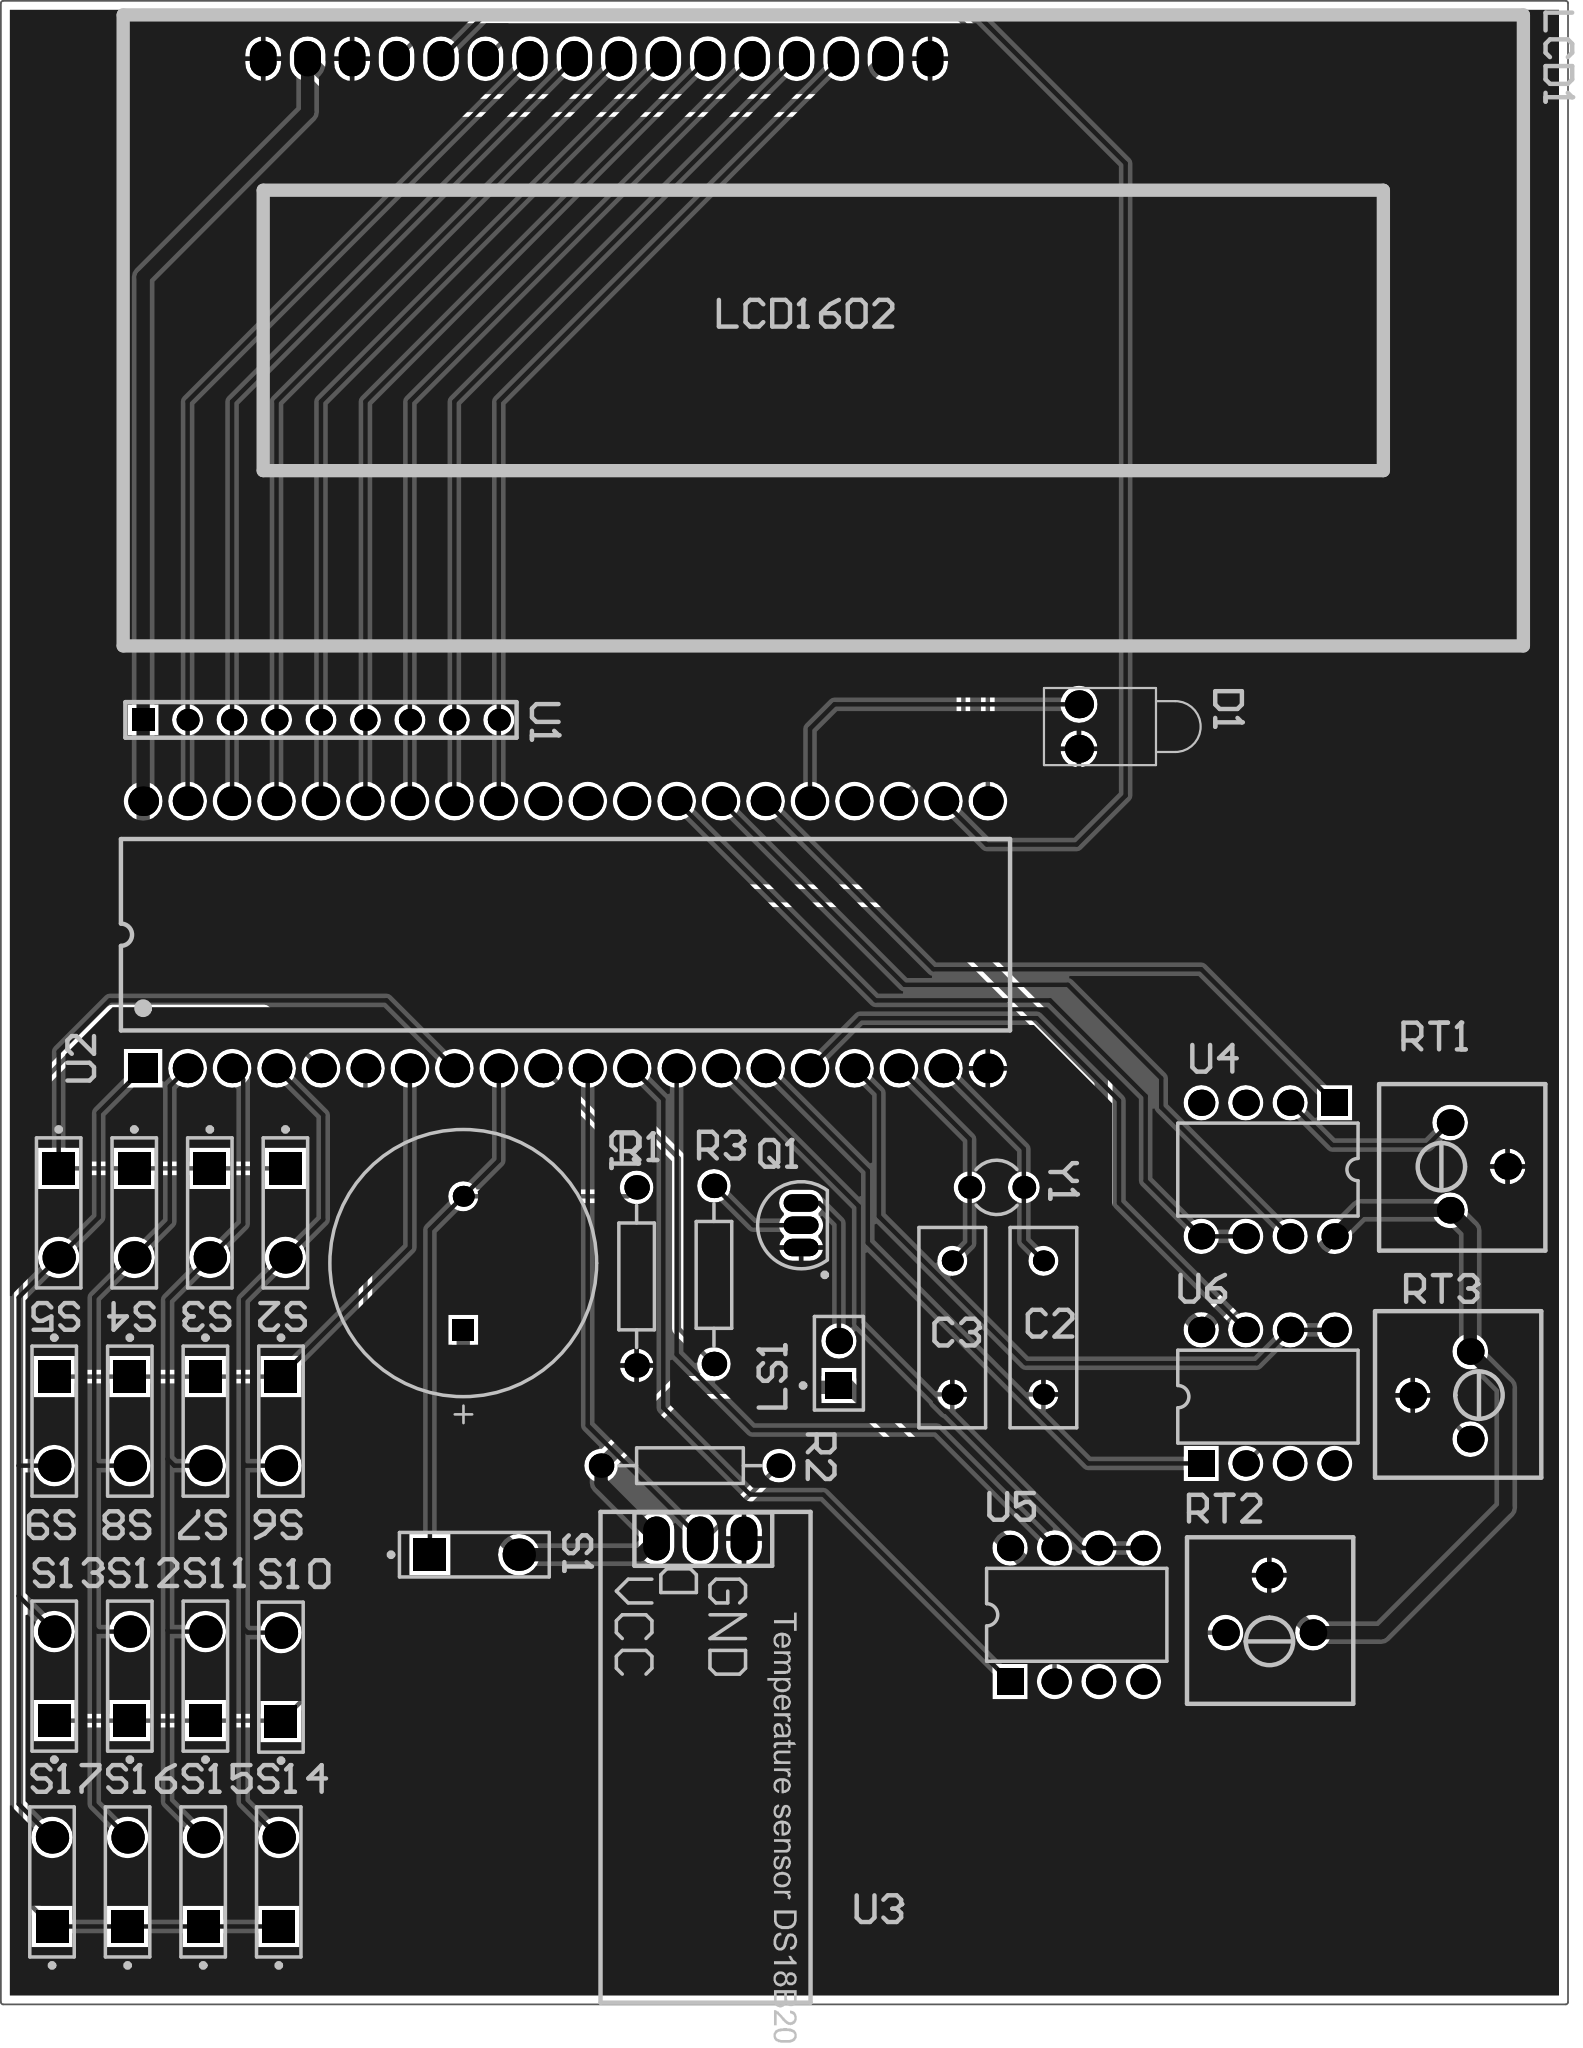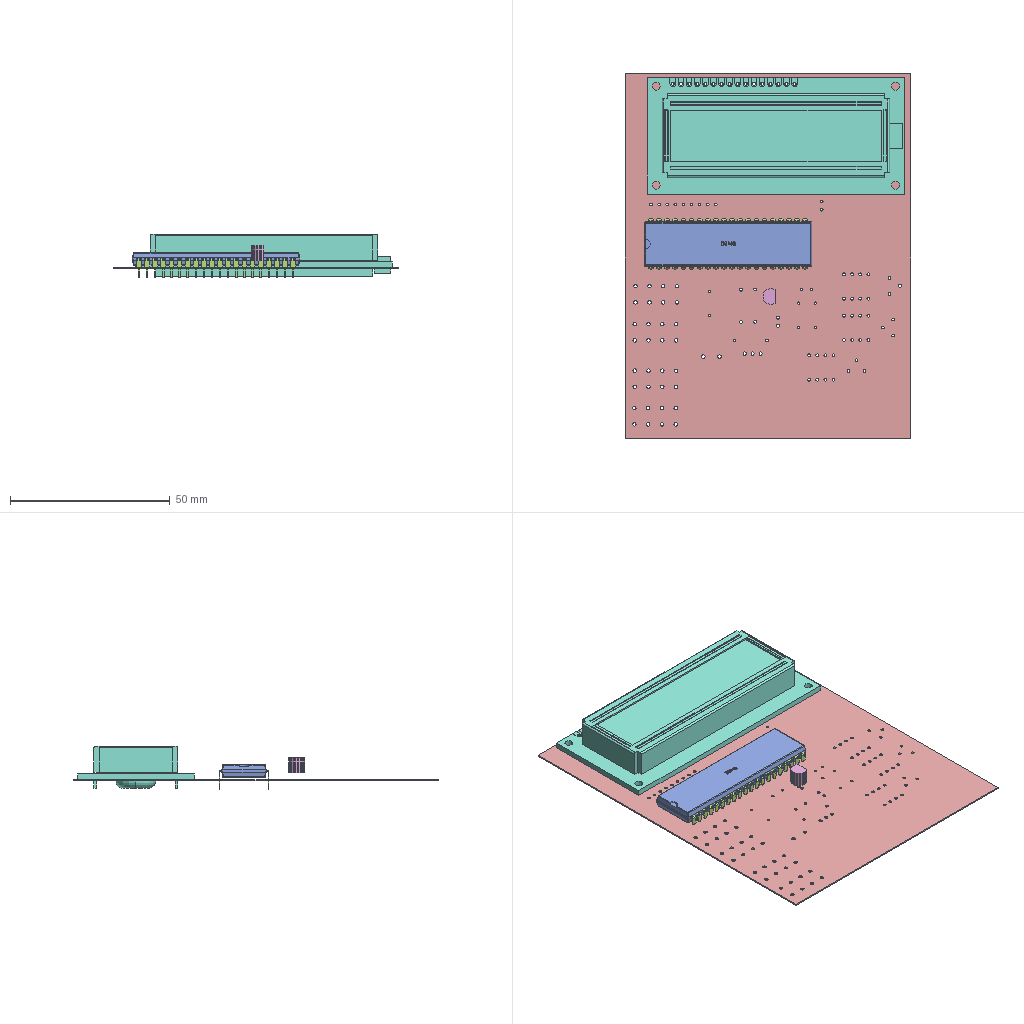Circuit board layout | Altium Designer | box 89.5 x 114.3 x 13.7 mm
Layer stack:
# Altium Designer layer stack of  (unit mm; dielectric type: 0 none, 1 core, 2 prepreg, 3 surface material)
index,name,kind,layer,copper_thickness_mm,dielectric_type,dielectric_thickness_mm,dielectric_material,dielectric_constant
0,Top Paste,other,,,,,,
1,Top Overlay,other,,,,,,
2,Top Solder,dielectric,,,3,0.0102,Solder Resist,3.5
3,Top Layer,copper,Top Layer,0.0356,,,,
4,Dielectric 1,dielectric,,,0,0.32,FR-4,4.8
5,Bottom Layer,copper,Bottom Layer,0.0356,,,,
6,Bottom Solder,dielectric,,,3,0.0102,Solder Resist,3.5
7,Bottom Overlay,other,,,,,,
8,Bottom Paste,other,,,,,,
# drill layer pairs: low layer,high layer
drill_pair,Top Layer,Bottom Layer
Part placement:
Designator,Comment,Layer,Footprint,Center-X(mm),Center-Y(mm),Rotation
Y1,12MHZ,TopLayer,R38,109.093,59.436,270
U6,ADC0832CCN,TopLayer,N08E,124.587,47.498,0
U5,ADC0832CCN,TopLayer,N08E,113.665,35.052,0
U4,ADC0832CCN,TopLayer,N08E,124.587,60.452,180
U3,DS18B20,TopLayer,DS18B20,92.154,39.404,270
U2,AT89C52,TopLayer,DIP40,84.455,73.85,90
U1,Resistor network,TopLayer,paizu,70.485,86.106,360
S17,SW-PB,TopLayer,SPST-2,55.118,19.812,90
S16,SW-PB,TopLayer,SPST-2,59.436,19.812,90
S15,SW-PB,TopLayer,SPST-2,63.754,19.812,90
S14,SW-PB,TopLayer,SPST-2,68.072,19.812,90
S13,SW-PB,TopLayer,SPST-2,55.245,31.554,90
S12,SW-PB,TopLayer,SPST-2,59.563,31.554,90
S11,SW-PB,TopLayer,SPST-2,63.881,31.554,90
S10,SW-PB,TopLayer,SPST-2,68.199,31.496,90
S9,SW-PB,TopLayer,SPST-2,55.245,46.101,270
S8,SW-PB,TopLayer,SPST-2,59.563,46.101,270
S7,SW-PB,TopLayer,SPST-2,63.881,46.101,270
S6,SW-PB,TopLayer,SPST-2,68.199,46.101,270
S5,SW-PB,TopLayer,SPST-2,55.499,57.981,270
S4,SW-PB,TopLayer,SPST-2,59.817,57.981,270
S3,SW-PB,TopLayer,SPST-2,64.135,57.981,270
S2,SW-PB,TopLayer,SPST-2,68.453,57.981,270
S1,SW-PB,TopLayer,SPST-2,79.248,38.481,360
RT3,1K,TopLayer,电位器,134.506,47.574,90
RT2,1K,TopLayer,电位器,124.663,35.674,360
RT1,1K,TopLayer,电位器,136.639,60.63,270
R3,1K,TopLayer,AXIAL-0.4,92.937,54.443,90
R2,1K,TopLayer,AXIAL-0.4,91.567,43.561,360
R1,1K,TopLayer,AXIAL-0.4,88.519,54.356,90
Q1,2N3904,TopLayer,TO-92A,97.917,57.277,0
LS1,Speaker,TopLayer,PIN2,100.076,49.403,90
LCD1,LCD1602,TopLayer,LCD1602,86.233,123.825,360
D1,LED1,TopLayer,LED-1,113.792,85.725,360
C3,22PF,TopLayer,RAD-0.3,106.553,51.435,90
C2,22PF,TopLayer,RAD-0.3,111.76,51.435,90
C1,1UF,TopLayer,RB7.6-15,78.613,55.118,270
Pad and via stacks:
# Altium Designer via and pad stacks of  (unit mm). Each distinct definition once, with the count of objects using it.
# via: kind,start_layer,end_layer,hole_mm,diameter_mm,mode(0 simple;1 top-mid-bottom;2 full stack),diameter_per_layer,count,example_net
# pad: kind,layer,hole_mm,hole_type(0 round;1 square;2 slot),plating,top_size,top_shape(1 round;2 rect;3 octagon;9 rounded rect),mid_size,bottom_size,mode,footprint,size_per_layer,count,example
pad,Multi-Layer,0.8,0,plated,1.6x1.6,1,1.6x1.6,1.6x1.6,0,LED-1,,2,D1.1
pad,Multi-Layer,0.84,0,plated,1.26x1.26,2,1.26x1.26,1.26x1.26,0,paizu,,1,U1.1
pad,Multi-Layer,0.84,0,plated,1.26x1.26,1,1.26x1.26,1.26x1.26,0,paizu,,8,U1.2
pad,Multi-Layer,0.8,0,plated,1.7x1.7,1,1.7x1.7,1.7x1.7,0,DIP40,,39,U2.21
pad,Multi-Layer,0.8,0,plated,1.7x1.7,2,1.7x1.7,1.7x1.7,0,DIP40,,1,U2.1
pad,Multi-Layer,0.9,0,plated,1.524x2.032,1,1.524x2.032,1.524x2.032,0,LCD1602,,16,LCD1.1
pad,Multi-Layer,1.1,0,plated,1.85x1.85,2,1.85x1.85,1.85x1.85,0,SPST-2,,17,S1.1
pad,Multi-Layer,1.1,0,plated,1.85x1.85,1,1.85x1.85,1.85x1.85,0,SPST-2,,17,S1.2
pad,Multi-Layer,0.7,0,plated,1.2x1.2,2,1.2x1.2,1.2x1.2,0,RB7.6-15,,1,C1.1
pad,Multi-Layer,0.7,0,plated,1.2x1.2,1,1.2x1.2,1.2x1.2,0,RB7.6-15,,1,C1.2
pad,Multi-Layer,0.85,0,plated,1.4x1.4,1,1.4x1.4,1.4x1.4,0,AXIAL-0.4,,6,R1.1
pad,Multi-Layer,0.7,0,plated,1.2x1.2,1,1.2x1.2,1.2x1.2,0,RAD-0.3,,4,C2.2
pad,Multi-Layer,0.7,0,plated,1.3x1.3,1,1.3x1.3,1.3x1.3,0,R38,,2,Y1.1
pad,Multi-Layer,0.9,0,plated,1.5x1.5,2,1.5x1.5,1.5x1.5,0,PIN2,,1,LS1.1
pad,Multi-Layer,0.9,0,plated,1.5x1.5,1,1.5x1.5,1.5x1.5,0,PIN2,,1,LS1.2
pad,Multi-Layer,0.9,2,plated,2.524x1.524,1,2.524x1.524,2.524x1.524,0,DS18B20,,3,U3.2
pad,Multi-Layer,0.9,0,plated,2x1,1,2x1,2x1,0,TO-92A,,3,Q1.3
pad,Multi-Layer,0.9,0,plated,1.5x1.5,2,1.5x1.5,1.5x1.5,0,N08E,,3,U5.1
pad,Multi-Layer,0.9,0,plated,1.5x1.5,1,1.5x1.5,1.5x1.5,0,N08E,,21,U5.2
pad,Multi-Layer,0.9,0,plated,1.524x1.524,1,1.524x1.524,1.524x1.524,0,\u00B5\u00E7\u00CE\u00BB\u00C6\u00F7,,9,RT2.2
Copper pours:
name,layer,net,type(0 solid;1 hatched;2 none)
G,Bottom Layer,GND,0
G,Top Layer,GND,0
Design rules, without the lines most boards share:
# Altium Designer design rules of  (exported by Altium Designer, unit mm)
# columns: name | kind | enabled | priority | scope1 | scope2 | descriptor | typed fields (field=value)
SilkToSilkClearance | 55 | enabled | 1 | All | All | Silk to Silk (Clearance=0mil) (All),(All) |
SilkToSolderMaskClearance | 54 | enabled | 1 | IsPad | All | Silk To Solder Mask (Clearance=0mil) (IsPad),(All) |
MinimumSolderMaskSliver | 53 | enabled | 1 | All | All | Minimum Solder Mask Sliver (Gap=0mil) (All),(All) |
HoleToHoleClearance | 52 | enabled | 1 | All | All | Hole To Hole Clearance (Gap=10mil) (All),(All) | gap=0.254
DiffPairsRouting | 51 | enabled | 1 | All | All | Differential Pairs Uncoupled Length using the Gap Constraints (Min=10mil) (Max=10mil) (Prefered=10mil)  and Width Constraints (Min=15mil) (Max=15mil) (Prefered=15mil) (All) |
SolderMaskExpansion | 13 | enabled | 1 | All | All | Solder Mask Expansion (Expansion =4mil) (All) | expansion=0.1016
PasteMaskExpansion | 14 | enabled | 1 | All | All | Paste Mask Expansion (Expansion =0mil) (All) | expansion=0
RoutingVias | 11 | enabled | 1 | All | All | Routing Via (MinHoleWidth=28mil) (MaxHoleWidth=28mil) (PreferredHoleWidth=28mil) (MinWidth=50mil) (MaxWidth=50mil) (PreferedWidth=50mil) (All) | via_min_hole=0.7112 via_max_hole=0.7112 via_preferred_diameter=1.27 via_preferred_hole=0.7112
Width | 2 | enabled | 1 | All | All | Width Constraint (Min=10mil) (Max=30mil) (Preferred=10mil) (All) |
PolygonConnect | 20 | enabled | 1 | All | All | Polygon Connect Rule(Relief Connect )(Conductor Width=10mil) (Relief Angle=90 Angle) (Entries=4) (Air Gap Width=10mil) (All),(All) | connect_style(0=relief,1=direct,2=none)=0 relief_conductor_width=0.254 relief_entries=4
PlaneConnect | 6 | enabled | 1 | All | All | Power Plane Connect Rule(Relief Connect )(Expansion=20mil) (Conductor Width=10mil) (Air Gap=10mil) (Entries=4) (All) | relief_conductor_width=0.254 relief_entries=4 relief_expansion=0.508
Clearance | 0 | enabled | 1 | All | All | Clearance Constraint (Gap=10mil) (All),(All) | gap=0.254
Classes set for this board:
# Altium Designer classes of  (member kind: 0 net, 1 component, 2 from-to, 3 pad, 4 layer, 5 differential pair, 6 design channel, 7 polygon, 8 structure, 9 xSignal)
# columns: class name | member kind | superclass | members
Sheet1 | 1 | no | C1; C2; C3; D1; LCD1; LS1; Q1; R1; R2; R3; RT1; RT2; RT3; S1; S2; S3; S4; S5; S6; S7; S8; S9; S10; S11; S12; S13; S14; S15; S16; S17; U1; U2; U3; U4; U5; U6; Y1;